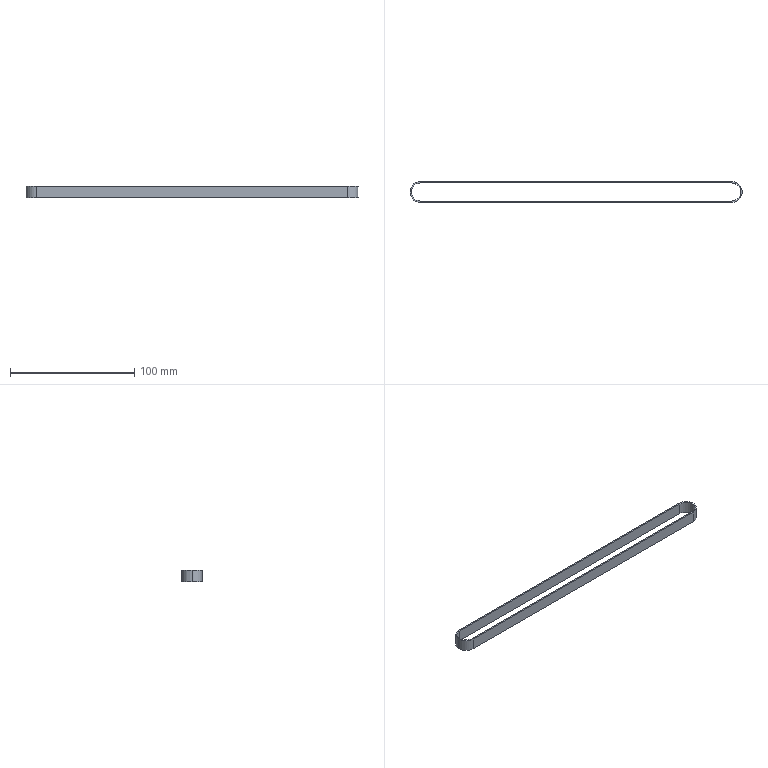Part | NX | features BREP 1 | 1 solid | 12 faces | box 267.76 x 16.76 x 9.5 mm | volume 5760 mm3 | plane 6 | cylinder 6 | commonest cylinder face diameters 14.56 x3 16.76 x3
STEP:
#1=CARTESIAN_POINT('',(251.,7.28,-4.75));
#2=VERTEX_POINT('',#1);
#3=CARTESIAN_POINT('',(0.,7.28,-4.75));
#4=VERTEX_POINT('',#3);
#5=CARTESIAN_POINT('',(0.,7.28,-4.75));
#6=DIRECTION('',(-1.,0.,0.));
#7=VECTOR('',#6,1000.);
#8=LINE('',#5,#7);
#9=EDGE_CURVE('',#2,#4,#8,.T.);
#10=ORIENTED_EDGE('',*,*,#9,.F.);
#11=CARTESIAN_POINT('',(251.,7.28,4.75));
#12=VERTEX_POINT('',#11);
#13=CARTESIAN_POINT('',(251.,7.28,4.75));
#14=DIRECTION('',(0.,0.,-1.));
#15=VECTOR('',#14,1000.);
#16=LINE('',#13,#15);
#17=EDGE_CURVE('',#12,#2,#16,.T.);
#18=ORIENTED_EDGE('',*,*,#17,.F.);
#19=CARTESIAN_POINT('',(0.,7.28,4.75));
#20=VERTEX_POINT('',#19);
#21=CARTESIAN_POINT('',(0.,7.28,4.75));
#22=DIRECTION('',(-1.,0.,0.));
#23=VECTOR('',#22,1000.);
#24=LINE('',#21,#23);
#25=EDGE_CURVE('',#12,#20,#24,.T.);
#26=ORIENTED_EDGE('',*,*,#25,.T.);
#27=CARTESIAN_POINT('',(0.,7.28,4.75));
#28=DIRECTION('',(0.,0.,-1.));
#29=VECTOR('',#28,1000.);
#30=LINE('',#27,#29);
#31=EDGE_CURVE('',#20,#4,#30,.T.);
#32=ORIENTED_EDGE('',*,*,#31,.T.);
#33=EDGE_LOOP('',(#10,#18,#26,#32));
#34=FACE_BOUND('',#33,.T.);
#35=CARTESIAN_POINT('',(0.,7.28,4.75));
#36=DIRECTION('',(0.,-1.,0.));
#37=DIRECTION('',(0.,0.,-1.));
#38=AXIS2_PLACEMENT_3D('',#35,#36,#37);
#39=PLANE('',#38);
#40=ADVANCED_FACE('',(#34),#39,.T.);
#41=CARTESIAN_POINT('',(251.,-7.28,-4.75));
#42=VERTEX_POINT('',#41);
#43=CARTESIAN_POINT('',(251.,0.,-4.75));
#44=DIRECTION('',(0.,0.,1.));
#45=DIRECTION('',(-1.,0.,0.));
#46=AXIS2_PLACEMENT_3D('',#43,#44,#45);
#47=CIRCLE('',#46,7.28);
#48=EDGE_CURVE('',#42,#2,#47,.T.);
#49=ORIENTED_EDGE('',*,*,#48,.F.);
#50=CARTESIAN_POINT('',(251.,-7.28,4.75));
#51=VERTEX_POINT('',#50);
#52=CARTESIAN_POINT('',(251.,-7.28,4.75));
#53=DIRECTION('',(0.,0.,-1.));
#54=VECTOR('',#53,1000.);
#55=LINE('',#52,#54);
#56=EDGE_CURVE('',#51,#42,#55,.T.);
#57=ORIENTED_EDGE('',*,*,#56,.F.);
#58=CARTESIAN_POINT('',(251.,0.,4.75));
#59=DIRECTION('',(0.,0.,1.));
#60=DIRECTION('',(-1.,0.,0.));
#61=AXIS2_PLACEMENT_3D('',#58,#59,#60);
#62=CIRCLE('',#61,7.28);
#63=EDGE_CURVE('',#51,#12,#62,.T.);
#64=ORIENTED_EDGE('',*,*,#63,.T.);
#65=ORIENTED_EDGE('',*,*,#17,.T.);
#66=EDGE_LOOP('',(#49,#57,#64,#65));
#67=FACE_BOUND('',#66,.T.);
#68=CARTESIAN_POINT('',(251.,0.,4.75));
#69=DIRECTION('',(0.,0.,-1.));
#70=DIRECTION('',(-1.,0.,0.));
#71=AXIS2_PLACEMENT_3D('',#68,#69,#70);
#72=CYLINDRICAL_SURFACE('',#71,7.28);
#73=ADVANCED_FACE('',(#67),#72,.F.);
#74=CARTESIAN_POINT('',(0.,-7.28,-4.75));
#75=VERTEX_POINT('',#74);
#76=CARTESIAN_POINT('',(0.,-7.28,-4.75));
#77=DIRECTION('',(1.,0.,0.));
#78=VECTOR('',#77,1000.);
#79=LINE('',#76,#78);
#80=EDGE_CURVE('',#75,#42,#79,.T.);
#81=ORIENTED_EDGE('',*,*,#80,.F.);
#82=CARTESIAN_POINT('',(0.,-7.28,4.75));
#83=VERTEX_POINT('',#82);
#84=CARTESIAN_POINT('',(0.,-7.28,4.75));
#85=DIRECTION('',(0.,0.,-1.));
#86=VECTOR('',#85,1000.);
#87=LINE('',#84,#86);
#88=EDGE_CURVE('',#83,#75,#87,.T.);
#89=ORIENTED_EDGE('',*,*,#88,.F.);
#90=CARTESIAN_POINT('',(0.,-7.28,4.75));
#91=DIRECTION('',(1.,0.,0.));
#92=VECTOR('',#91,1000.);
#93=LINE('',#90,#92);
#94=EDGE_CURVE('',#83,#51,#93,.T.);
#95=ORIENTED_EDGE('',*,*,#94,.T.);
#96=ORIENTED_EDGE('',*,*,#56,.T.);
#97=EDGE_LOOP('',(#81,#89,#95,#96));
#98=FACE_BOUND('',#97,.T.);
#99=CARTESIAN_POINT('',(0.,-7.28,4.75));
#100=DIRECTION('',(0.,1.,0.));
#101=DIRECTION('',(0.,0.,1.));
#102=AXIS2_PLACEMENT_3D('',#99,#100,#101);
#103=PLANE('',#102);
#104=ADVANCED_FACE('',(#98),#103,.T.);
#105=CARTESIAN_POINT('',(-7.28,0.,4.75));
#106=VERTEX_POINT('',#105);
#107=CARTESIAN_POINT('',(-7.28,0.,-4.75));
#108=VERTEX_POINT('',#107);
#109=CARTESIAN_POINT('',(-7.28,0.,4.75));
#110=DIRECTION('',(0.,0.,-1.));
#111=VECTOR('',#110,1000.);
#112=LINE('',#109,#111);
#113=EDGE_CURVE('',#106,#108,#112,.T.);
#114=ORIENTED_EDGE('',*,*,#113,.F.);
#115=CARTESIAN_POINT('',(0.,0.,4.75));
#116=DIRECTION('',(0.,0.,1.));
#117=DIRECTION('',(-1.,0.,0.));
#118=AXIS2_PLACEMENT_3D('',#115,#116,#117);
#119=CIRCLE('',#118,7.28);
#120=EDGE_CURVE('',#106,#83,#119,.T.);
#121=ORIENTED_EDGE('',*,*,#120,.T.);
#122=ORIENTED_EDGE('',*,*,#88,.T.);
#123=CARTESIAN_POINT('',(0.,0.,-4.75));
#124=DIRECTION('',(0.,0.,1.));
#125=DIRECTION('',(-1.,0.,0.));
#126=AXIS2_PLACEMENT_3D('',#123,#124,#125);
#127=CIRCLE('',#126,7.28);
#128=EDGE_CURVE('',#108,#75,#127,.T.);
#129=ORIENTED_EDGE('',*,*,#128,.F.);
#130=EDGE_LOOP('',(#114,#121,#122,#129));
#131=FACE_BOUND('',#130,.T.);
#132=CARTESIAN_POINT('',(0.,0.,4.75));
#133=DIRECTION('',(0.,0.,-1.));
#134=DIRECTION('',(-1.,0.,0.));
#135=AXIS2_PLACEMENT_3D('',#132,#133,#134);
#136=CYLINDRICAL_SURFACE('',#135,7.28);
#137=ADVANCED_FACE('',(#131),#136,.F.);
#138=CARTESIAN_POINT('',(251.,8.38,-4.75));
#139=VERTEX_POINT('',#138);
#140=CARTESIAN_POINT('',(0.,8.38,-4.75));
#141=VERTEX_POINT('',#140);
#142=CARTESIAN_POINT('',(0.,8.38,-4.75));
#143=DIRECTION('',(-1.,0.,0.));
#144=VECTOR('',#143,1000.);
#145=LINE('',#142,#144);
#146=EDGE_CURVE('',#139,#141,#145,.T.);
#147=ORIENTED_EDGE('',*,*,#146,.T.);
#148=CARTESIAN_POINT('',(0.,8.38,4.75));
#149=VERTEX_POINT('',#148);
#150=CARTESIAN_POINT('',(0.,8.38,4.75));
#151=DIRECTION('',(0.,0.,-1.));
#152=VECTOR('',#151,1000.);
#153=LINE('',#150,#152);
#154=EDGE_CURVE('',#149,#141,#153,.T.);
#155=ORIENTED_EDGE('',*,*,#154,.F.);
#156=CARTESIAN_POINT('',(251.,8.38,4.75));
#157=VERTEX_POINT('',#156);
#158=CARTESIAN_POINT('',(0.,8.38,4.75));
#159=DIRECTION('',(-1.,0.,0.));
#160=VECTOR('',#159,1000.);
#161=LINE('',#158,#160);
#162=EDGE_CURVE('',#157,#149,#161,.T.);
#163=ORIENTED_EDGE('',*,*,#162,.F.);
#164=CARTESIAN_POINT('',(251.,8.38,4.75));
#165=DIRECTION('',(0.,0.,-1.));
#166=VECTOR('',#165,1000.);
#167=LINE('',#164,#166);
#168=EDGE_CURVE('',#157,#139,#167,.T.);
#169=ORIENTED_EDGE('',*,*,#168,.T.);
#170=EDGE_LOOP('',(#147,#155,#163,#169));
#171=FACE_BOUND('',#170,.T.);
#172=CARTESIAN_POINT('',(0.,8.38,4.75));
#173=DIRECTION('',(0.,-1.,0.));
#174=DIRECTION('',(0.,0.,-1.));
#175=AXIS2_PLACEMENT_3D('',#172,#173,#174);
#176=PLANE('',#175);
#177=ADVANCED_FACE('',(#171),#176,.F.);
#178=CARTESIAN_POINT('',(251.,-8.38,-4.75));
#179=VERTEX_POINT('',#178);
#180=CARTESIAN_POINT('',(251.,0.,-4.75));
#181=DIRECTION('',(0.,0.,1.));
#182=DIRECTION('',(-1.,0.,0.));
#183=AXIS2_PLACEMENT_3D('',#180,#181,#182);
#184=CIRCLE('',#183,8.38);
#185=EDGE_CURVE('',#179,#139,#184,.T.);
#186=ORIENTED_EDGE('',*,*,#185,.T.);
#187=ORIENTED_EDGE('',*,*,#168,.F.);
#188=CARTESIAN_POINT('',(251.,-8.38,4.75));
#189=VERTEX_POINT('',#188);
#190=CARTESIAN_POINT('',(251.,0.,4.75));
#191=DIRECTION('',(0.,0.,1.));
#192=DIRECTION('',(-1.,0.,0.));
#193=AXIS2_PLACEMENT_3D('',#190,#191,#192);
#194=CIRCLE('',#193,8.38);
#195=EDGE_CURVE('',#189,#157,#194,.T.);
#196=ORIENTED_EDGE('',*,*,#195,.F.);
#197=CARTESIAN_POINT('',(251.,-8.38,4.75));
#198=DIRECTION('',(0.,0.,-1.));
#199=VECTOR('',#198,1000.);
#200=LINE('',#197,#199);
#201=EDGE_CURVE('',#189,#179,#200,.T.);
#202=ORIENTED_EDGE('',*,*,#201,.T.);
#203=EDGE_LOOP('',(#186,#187,#196,#202));
#204=FACE_BOUND('',#203,.T.);
#205=CARTESIAN_POINT('',(251.,0.,4.75));
#206=DIRECTION('',(0.,0.,-1.));
#207=DIRECTION('',(-1.,0.,0.));
#208=AXIS2_PLACEMENT_3D('',#205,#206,#207);
#209=CYLINDRICAL_SURFACE('',#208,8.38);
#210=ADVANCED_FACE('',(#204),#209,.T.);
#211=CARTESIAN_POINT('',(0.,-8.38,-4.75));
#212=VERTEX_POINT('',#211);
#213=CARTESIAN_POINT('',(0.,-8.38,-4.75));
#214=DIRECTION('',(1.,0.,0.));
#215=VECTOR('',#214,1000.);
#216=LINE('',#213,#215);
#217=EDGE_CURVE('',#212,#179,#216,.T.);
#218=ORIENTED_EDGE('',*,*,#217,.T.);
#219=ORIENTED_EDGE('',*,*,#201,.F.);
#220=CARTESIAN_POINT('',(0.,-8.38,4.75));
#221=VERTEX_POINT('',#220);
#222=CARTESIAN_POINT('',(0.,-8.38,4.75));
#223=DIRECTION('',(1.,0.,0.));
#224=VECTOR('',#223,1000.);
#225=LINE('',#222,#224);
#226=EDGE_CURVE('',#221,#189,#225,.T.);
#227=ORIENTED_EDGE('',*,*,#226,.F.);
#228=CARTESIAN_POINT('',(0.,-8.38,4.75));
#229=DIRECTION('',(0.,0.,-1.));
#230=VECTOR('',#229,1000.);
#231=LINE('',#228,#230);
#232=EDGE_CURVE('',#221,#212,#231,.T.);
#233=ORIENTED_EDGE('',*,*,#232,.T.);
#234=EDGE_LOOP('',(#218,#219,#227,#233));
#235=FACE_BOUND('',#234,.T.);
#236=CARTESIAN_POINT('',(0.,-8.38,4.75));
#237=DIRECTION('',(0.,1.,0.));
#238=DIRECTION('',(0.,0.,1.));
#239=AXIS2_PLACEMENT_3D('',#236,#237,#238);
#240=PLANE('',#239);
#241=ADVANCED_FACE('',(#235),#240,.F.);
#242=CARTESIAN_POINT('',(-8.38,0.,4.75));
#243=VERTEX_POINT('',#242);
#244=CARTESIAN_POINT('',(-8.38,0.,-4.75));
#245=VERTEX_POINT('',#244);
#246=CARTESIAN_POINT('',(-8.38,0.,4.75));
#247=DIRECTION('',(0.,0.,-1.));
#248=VECTOR('',#247,1000.);
#249=LINE('',#246,#248);
#250=EDGE_CURVE('',#243,#245,#249,.T.);
#251=ORIENTED_EDGE('',*,*,#250,.F.);
#252=CARTESIAN_POINT('',(0.,0.,4.75));
#253=DIRECTION('',(0.,0.,1.));
#254=DIRECTION('',(-1.,0.,0.));
#255=AXIS2_PLACEMENT_3D('',#252,#253,#254);
#256=CIRCLE('',#255,8.38);
#257=EDGE_CURVE('',#149,#243,#256,.T.);
#258=ORIENTED_EDGE('',*,*,#257,.F.);
#259=ORIENTED_EDGE('',*,*,#154,.T.);
#260=CARTESIAN_POINT('',(0.,0.,-4.75));
#261=DIRECTION('',(0.,0.,1.));
#262=DIRECTION('',(-1.,0.,0.));
#263=AXIS2_PLACEMENT_3D('',#260,#261,#262);
#264=CIRCLE('',#263,8.38);
#265=EDGE_CURVE('',#141,#245,#264,.T.);
#266=ORIENTED_EDGE('',*,*,#265,.T.);
#267=EDGE_LOOP('',(#251,#258,#259,#266));
#268=FACE_BOUND('',#267,.T.);
#269=CARTESIAN_POINT('',(0.,0.,4.75));
#270=DIRECTION('',(0.,0.,-1.));
#271=DIRECTION('',(-1.,0.,0.));
#272=AXIS2_PLACEMENT_3D('',#269,#270,#271);
#273=CYLINDRICAL_SURFACE('',#272,8.38);
#274=ADVANCED_FACE('',(#268),#273,.T.);
#275=ORIENTED_EDGE('',*,*,#9,.T.);
#276=CARTESIAN_POINT('',(0.,0.,-4.75));
#277=DIRECTION('',(0.,0.,1.));
#278=DIRECTION('',(-1.,0.,0.));
#279=AXIS2_PLACEMENT_3D('',#276,#277,#278);
#280=CIRCLE('',#279,7.28);
#281=EDGE_CURVE('',#4,#108,#280,.T.);
#282=ORIENTED_EDGE('',*,*,#281,.T.);
#283=ORIENTED_EDGE('',*,*,#128,.T.);
#284=ORIENTED_EDGE('',*,*,#80,.T.);
#285=ORIENTED_EDGE('',*,*,#48,.T.);
#286=EDGE_LOOP('',(#275,#282,#283,#284,#285));
#287=FACE_BOUND('',#286,.T.);
#288=ORIENTED_EDGE('',*,*,#265,.F.);
#289=ORIENTED_EDGE('',*,*,#146,.F.);
#290=ORIENTED_EDGE('',*,*,#185,.F.);
#291=ORIENTED_EDGE('',*,*,#217,.F.);
#292=CARTESIAN_POINT('',(0.,0.,-4.75));
#293=DIRECTION('',(0.,0.,1.));
#294=DIRECTION('',(-1.,0.,0.));
#295=AXIS2_PLACEMENT_3D('',#292,#293,#294);
#296=CIRCLE('',#295,8.38);
#297=EDGE_CURVE('',#245,#212,#296,.T.);
#298=ORIENTED_EDGE('',*,*,#297,.F.);
#299=EDGE_LOOP('',(#288,#289,#290,#291,#298));
#300=FACE_BOUND('',#299,.T.);
#301=CARTESIAN_POINT('',(0.,0.,-4.75));
#302=DIRECTION('',(0.,0.,-1.));
#303=DIRECTION('',(-1.,0.,0.));
#304=AXIS2_PLACEMENT_3D('',#301,#302,#303);
#305=PLANE('',#304);
#306=ADVANCED_FACE('',(#287,#300),#305,.T.);
#307=CARTESIAN_POINT('',(0.,0.,4.75));
#308=DIRECTION('',(0.,0.,1.));
#309=DIRECTION('',(-1.,0.,0.));
#310=AXIS2_PLACEMENT_3D('',#307,#308,#309);
#311=CIRCLE('',#310,7.28);
#312=EDGE_CURVE('',#20,#106,#311,.T.);
#313=ORIENTED_EDGE('',*,*,#312,.F.);
#314=ORIENTED_EDGE('',*,*,#25,.F.);
#315=ORIENTED_EDGE('',*,*,#63,.F.);
#316=ORIENTED_EDGE('',*,*,#94,.F.);
#317=ORIENTED_EDGE('',*,*,#120,.F.);
#318=EDGE_LOOP('',(#313,#314,#315,#316,#317));
#319=FACE_BOUND('',#318,.T.);
#320=ORIENTED_EDGE('',*,*,#257,.T.);
#321=CARTESIAN_POINT('',(0.,0.,4.75));
#322=DIRECTION('',(0.,0.,1.));
#323=DIRECTION('',(-1.,0.,0.));
#324=AXIS2_PLACEMENT_3D('',#321,#322,#323);
#325=CIRCLE('',#324,8.38);
#326=EDGE_CURVE('',#243,#221,#325,.T.);
#327=ORIENTED_EDGE('',*,*,#326,.T.);
#328=ORIENTED_EDGE('',*,*,#226,.T.);
#329=ORIENTED_EDGE('',*,*,#195,.T.);
#330=ORIENTED_EDGE('',*,*,#162,.T.);
#331=EDGE_LOOP('',(#320,#327,#328,#329,#330));
#332=FACE_BOUND('',#331,.T.);
#333=CARTESIAN_POINT('',(0.,0.,4.75));
#334=DIRECTION('',(0.,0.,-1.));
#335=DIRECTION('',(-1.,0.,0.));
#336=AXIS2_PLACEMENT_3D('',#333,#334,#335);
#337=PLANE('',#336);
#338=ADVANCED_FACE('',(#319,#332),#337,.F.);
#339=ORIENTED_EDGE('',*,*,#326,.F.);
#340=ORIENTED_EDGE('',*,*,#250,.T.);
#341=ORIENTED_EDGE('',*,*,#297,.T.);
#342=ORIENTED_EDGE('',*,*,#232,.F.);
#343=EDGE_LOOP('',(#339,#340,#341,#342));
#344=FACE_BOUND('',#343,.T.);
#345=CARTESIAN_POINT('',(0.,0.,4.75));
#346=DIRECTION('',(0.,0.,-1.));
#347=DIRECTION('',(-1.,0.,0.));
#348=AXIS2_PLACEMENT_3D('',#345,#346,#347);
#349=CYLINDRICAL_SURFACE('',#348,8.38);
#350=ADVANCED_FACE('',(#344),#349,.T.);
#351=ORIENTED_EDGE('',*,*,#312,.T.);
#352=ORIENTED_EDGE('',*,*,#113,.T.);
#353=ORIENTED_EDGE('',*,*,#281,.F.);
#354=ORIENTED_EDGE('',*,*,#31,.F.);
#355=EDGE_LOOP('',(#351,#352,#353,#354));
#356=FACE_BOUND('',#355,.T.);
#357=CARTESIAN_POINT('',(0.,0.,4.75));
#358=DIRECTION('',(0.,0.,-1.));
#359=DIRECTION('',(-1.,0.,0.));
#360=AXIS2_PLACEMENT_3D('',#357,#358,#359);
#361=CYLINDRICAL_SURFACE('',#360,7.28);
#362=ADVANCED_FACE('',(#356),#361,.F.);
#363=CLOSED_SHELL('',(#40,#73,#104,#137,#177,#210,#241,#274,#306,#338,#350,#362));
#364=MANIFOLD_SOLID_BREP('',#363);
#365=(LENGTH_UNIT()NAMED_UNIT(*)SI_UNIT(.MILLI.,.METRE.));
#366=UNCERTAINTY_MEASURE_WITH_UNIT(LENGTH_MEASURE(0.00001),#365,'','');
#367=(NAMED_UNIT(*)PLANE_ANGLE_UNIT()SI_UNIT($,.RADIAN.));
#368=(NAMED_UNIT(*)SI_UNIT($,.STERADIAN.)SOLID_ANGLE_UNIT());
#369=(GEOMETRIC_REPRESENTATION_CONTEXT(3)GLOBAL_UNCERTAINTY_ASSIGNED_CONTEXT((#366))GLOBAL_UNIT_ASSIGNED_CONTEXT((#365,#367,#368))REPRESENTATION_CONTEXT('',''));
#370=ADVANCED_BREP_SHAPE_REPRESENTATION('',(#364),#369);